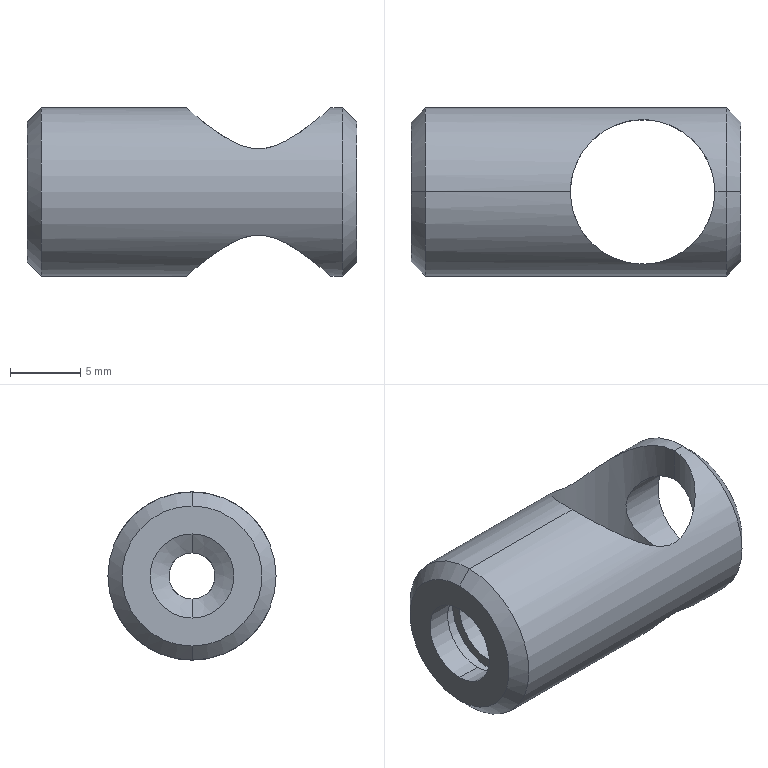Part | SolidWorks | features BaseBody 1 | 1 solid | 24 faces | box 23.5 x 12 x 12 mm | volume 1412 mm3 | cylinder 14 | cone 6 | plane 4 | commonest cylinder face diameters 6 x4 3.3 x2 7 x2 7.4 x2 10.3 x2 12 x2
STEP:
#1=CARTESIAN_POINT('',(486.537,37.715,59.366));
#2=VERTEX_POINT('',#1);
#3=CARTESIAN_POINT('',(486.537,37.715,71.366));
#4=VERTEX_POINT('',#3);
#5=CARTESIAN_POINT('',(486.537,37.715,65.366));
#6=DIRECTION('',(1.,0.,0.000000013));
#7=DIRECTION('',(0.,1.,0.));
#8=AXIS2_PLACEMENT_3D('',#5,#6,#7);
#9=CIRCLE('',#8,6.);
#10=EDGE_CURVE('',#2,#4,#9,.T.);
#11=ORIENTED_EDGE('',*,*,#10,.F.);
#12=CARTESIAN_POINT('',(485.687,37.715,59.366));
#13=VERTEX_POINT('',#12);
#14=CARTESIAN_POINT('',(486.537,37.715,59.366));
#15=DIRECTION('',(-1.,0.,-0.000000013));
#16=VECTOR('',#15,1000.);
#17=LINE('',#14,#16);
#18=EDGE_CURVE('',#2,#13,#17,.T.);
#19=ORIENTED_EDGE('',*,*,#18,.T.);
#20=CARTESIAN_POINT('',(475.387,37.715,59.366));
#21=VERTEX_POINT('',#20);
#22=CARTESIAN_POINT('',(475.387,37.715,59.366));
#23=CARTESIAN_POINT('',(475.387,37.895,59.366));
#24=CARTESIAN_POINT('',(475.396,38.075,59.374));
#25=CARTESIAN_POINT('',(475.434,38.436,59.407));
#26=CARTESIAN_POINT('',(475.463,38.616,59.431));
#27=CARTESIAN_POINT('',(475.538,38.965,59.495));
#28=CARTESIAN_POINT('',(475.584,39.136,59.534));
#29=CARTESIAN_POINT('',(475.692,39.47,59.626));
#30=CARTESIAN_POINT('',(475.755,39.634,59.679));
#31=CARTESIAN_POINT('',(475.964,40.108,59.854));
#32=CARTESIAN_POINT('',(476.129,40.399,59.991));
#33=CARTESIAN_POINT('',(476.509,40.941,60.297));
#34=CARTESIAN_POINT('',(476.72,41.187,60.465));
#35=CARTESIAN_POINT('',(477.174,41.628,60.809));
#36=CARTESIAN_POINT('',(477.418,41.825,60.988));
#37=CARTESIAN_POINT('',(477.945,42.176,61.346));
#38=CARTESIAN_POINT('',(478.225,42.328,61.524));
#39=CARTESIAN_POINT('',(478.67,42.517,61.768));
#40=CARTESIAN_POINT('',(478.824,42.574,61.846));
#41=CARTESIAN_POINT('',(479.142,42.675,61.989));
#42=CARTESIAN_POINT('',(479.309,42.719,62.055));
#43=CARTESIAN_POINT('',(479.647,42.79,62.165));
#44=CARTESIAN_POINT('',(479.821,42.818,62.21));
#45=CARTESIAN_POINT('',(480.178,42.855,62.272));
#46=CARTESIAN_POINT('',(480.362,42.865,62.288));
#47=CARTESIAN_POINT('',(480.913,42.864,62.286));
#48=CARTESIAN_POINT('',(481.268,42.824,62.218));
#49=CARTESIAN_POINT('',(481.949,42.679,61.994));
#50=CARTESIAN_POINT('',(482.263,42.578,61.845));
#51=CARTESIAN_POINT('',(482.858,42.323,61.518));
#52=CARTESIAN_POINT('',(483.139,42.17,61.34));
#53=CARTESIAN_POINT('',(483.66,41.822,60.985));
#54=CARTESIAN_POINT('',(483.903,41.625,60.807));
#55=CARTESIAN_POINT('',(484.358,41.182,60.461));
#56=CARTESIAN_POINT('',(484.57,40.933,60.293));
#57=CARTESIAN_POINT('',(484.946,40.396,59.99));
#58=CARTESIAN_POINT('',(485.111,40.106,59.853));
#59=CARTESIAN_POINT('',(485.39,39.471,59.619));
#60=CARTESIAN_POINT('',(485.499,39.139,59.527));
#61=CARTESIAN_POINT('',(485.611,38.615,59.431));
#62=CARTESIAN_POINT('',(485.639,38.435,59.407));
#63=CARTESIAN_POINT('',(485.677,38.075,59.374));
#64=CARTESIAN_POINT('',(485.687,37.895,59.366));
#65=CARTESIAN_POINT('',(485.687,37.715,59.366));
#66=B_SPLINE_CURVE_WITH_KNOTS('',3,(#22,#23,#24,#25,#26,#27,#28,#29,#30,#31,#32,#33,#34,#35,#36,#37,#38,#39,#40,#41,#42,#43,#44,#45,#46,#47,#48,#49,#50,#51,#52,#53,#54,#55,#56,#57,#58,#59,#60,#61,#62,#63,#64,#65),.UNSPECIFIED.,.F.,.F.,(4,2,2,2,2,2,2,2,2,2,2,2,2,2,2,2,2,2,2,2,2,4),(0.008683,0.009225,0.009768,0.01031,0.01085,0.01194,0.01302,0.01411,0.01519,0.01573,0.01627,0.01682,0.01736,0.01844,0.01953,0.02061,0.0217,0.02278,0.02387,0.02495,0.02549,0.02604),.UNSPECIFIED.);
#67=EDGE_CURVE('',#21,#13,#66,.T.);
#68=ORIENTED_EDGE('',*,*,#67,.F.);
#69=CARTESIAN_POINT('',(465.037,37.715,59.366));
#70=VERTEX_POINT('',#69);
#71=CARTESIAN_POINT('',(486.537,37.715,59.366));
#72=DIRECTION('',(-1.,0.,-0.000000013));
#73=VECTOR('',#72,1000.);
#74=LINE('',#71,#73);
#75=EDGE_CURVE('',#21,#70,#74,.T.);
#76=ORIENTED_EDGE('',*,*,#75,.T.);
#77=CARTESIAN_POINT('',(465.037,37.715,71.366));
#78=VERTEX_POINT('',#77);
#79=CARTESIAN_POINT('',(465.037,37.715,65.366));
#80=DIRECTION('',(-1.,0.,-0.000000013));
#81=DIRECTION('',(0.,1.,0.));
#82=AXIS2_PLACEMENT_3D('',#79,#80,#81);
#83=CIRCLE('',#82,6.);
#84=EDGE_CURVE('',#78,#70,#83,.T.);
#85=ORIENTED_EDGE('',*,*,#84,.F.);
#86=CARTESIAN_POINT('',(475.387,37.715,71.366));
#87=VERTEX_POINT('',#86);
#88=CARTESIAN_POINT('',(486.537,37.715,71.366));
#89=DIRECTION('',(-1.,0.,-0.000000013));
#90=VECTOR('',#89,1000.);
#91=LINE('',#88,#90);
#92=EDGE_CURVE('',#87,#78,#91,.T.);
#93=ORIENTED_EDGE('',*,*,#92,.F.);
#94=CARTESIAN_POINT('',(485.687,37.715,71.366));
#95=VERTEX_POINT('',#94);
#96=CARTESIAN_POINT('',(485.687,37.715,71.366));
#97=CARTESIAN_POINT('',(485.687,37.895,71.366));
#98=CARTESIAN_POINT('',(485.677,38.075,71.358));
#99=CARTESIAN_POINT('',(485.639,38.436,71.325));
#100=CARTESIAN_POINT('',(485.611,38.616,71.301));
#101=CARTESIAN_POINT('',(485.536,38.965,71.237));
#102=CARTESIAN_POINT('',(485.49,39.136,71.198));
#103=CARTESIAN_POINT('',(485.382,39.47,71.106));
#104=CARTESIAN_POINT('',(485.319,39.634,71.053));
#105=CARTESIAN_POINT('',(485.11,40.108,70.878));
#106=CARTESIAN_POINT('',(484.944,40.399,70.741));
#107=CARTESIAN_POINT('',(484.565,40.941,70.435));
#108=CARTESIAN_POINT('',(484.354,41.187,70.267));
#109=CARTESIAN_POINT('',(483.9,41.628,69.923));
#110=CARTESIAN_POINT('',(483.656,41.825,69.744));
#111=CARTESIAN_POINT('',(483.129,42.176,69.386));
#112=CARTESIAN_POINT('',(482.849,42.328,69.208));
#113=CARTESIAN_POINT('',(482.403,42.517,68.964));
#114=CARTESIAN_POINT('',(482.25,42.574,68.886));
#115=CARTESIAN_POINT('',(481.931,42.675,68.743));
#116=CARTESIAN_POINT('',(481.765,42.719,68.677));
#117=CARTESIAN_POINT('',(481.426,42.79,68.566));
#118=CARTESIAN_POINT('',(481.253,42.818,68.522));
#119=CARTESIAN_POINT('',(480.896,42.855,68.46));
#120=CARTESIAN_POINT('',(480.712,42.865,68.444));
#121=CARTESIAN_POINT('',(480.16,42.864,68.446));
#122=CARTESIAN_POINT('',(479.805,42.824,68.514));
#123=CARTESIAN_POINT('',(479.124,42.679,68.738));
#124=CARTESIAN_POINT('',(478.811,42.578,68.886));
#125=CARTESIAN_POINT('',(478.216,42.323,69.213));
#126=CARTESIAN_POINT('',(477.935,42.17,69.392));
#127=CARTESIAN_POINT('',(477.414,41.822,69.747));
#128=CARTESIAN_POINT('',(477.171,41.625,69.925));
#129=CARTESIAN_POINT('',(476.715,41.182,70.271));
#130=CARTESIAN_POINT('',(476.503,40.933,70.439));
#131=CARTESIAN_POINT('',(476.128,40.396,70.742));
#132=CARTESIAN_POINT('',(475.962,40.106,70.879));
#133=CARTESIAN_POINT('',(475.683,39.471,71.113));
#134=CARTESIAN_POINT('',(475.575,39.139,71.205));
#135=CARTESIAN_POINT('',(475.463,38.615,71.301));
#136=CARTESIAN_POINT('',(475.434,38.435,71.325));
#137=CARTESIAN_POINT('',(475.396,38.075,71.358));
#138=CARTESIAN_POINT('',(475.387,37.895,71.366));
#139=CARTESIAN_POINT('',(475.387,37.715,71.366));
#140=B_SPLINE_CURVE_WITH_KNOTS('',3,(#96,#97,#98,#99,#100,#101,#102,#103,#104,#105,#106,#107,#108,#109,#110,#111,#112,#113,#114,#115,#116,#117,#118,#119,#120,#121,#122,#123,#124,#125,#126,#127,#128,#129,#130,#131,#132,#133,#134,#135,#136,#137,#138,#139),.UNSPECIFIED.,.F.,.F.,(4,2,2,2,2,2,2,2,2,2,2,2,2,2,2,2,2,2,2,2,2,4),(0.008683,0.009225,0.009768,0.01031,0.01085,0.01194,0.01302,0.01411,0.01519,0.01573,0.01627,0.01682,0.01736,0.01844,0.01953,0.02061,0.0217,0.02278,0.02387,0.02495,0.02549,0.02604),.UNSPECIFIED.);
#141=EDGE_CURVE('',#95,#87,#140,.T.);
#142=ORIENTED_EDGE('',*,*,#141,.F.);
#143=CARTESIAN_POINT('',(486.537,37.715,71.366));
#144=DIRECTION('',(-1.,0.,-0.000000013));
#145=VECTOR('',#144,1000.);
#146=LINE('',#143,#145);
#147=EDGE_CURVE('',#4,#95,#146,.T.);
#148=ORIENTED_EDGE('',*,*,#147,.F.);
#149=EDGE_LOOP('',(#11,#19,#68,#76,#85,#93,#142,#148));
#150=FACE_OUTER_BOUND('',#149,.T.);
#151=CARTESIAN_POINT('',(486.537,37.715,65.366));
#152=DIRECTION('',(-1.,0.,-0.000000013));
#153=DIRECTION('',(-0.000000013,0.,1.));
#154=AXIS2_PLACEMENT_3D('',#151,#152,#153);
#155=CYLINDRICAL_SURFACE('',#154,6.);
#156=ADVANCED_FACE('',(#150),#155,.T.);
#157=CARTESIAN_POINT('',(487.537,37.715,60.366));
#158=VERTEX_POINT('',#157);
#159=CARTESIAN_POINT('',(487.537,37.715,70.366));
#160=VERTEX_POINT('',#159);
#161=CARTESIAN_POINT('',(487.537,37.715,65.366));
#162=DIRECTION('',(1.,0.,0.000000013));
#163=DIRECTION('',(-0.000000013,0.,1.));
#164=AXIS2_PLACEMENT_3D('',#161,#162,#163);
#165=CIRCLE('',#164,5.);
#166=EDGE_CURVE('',#158,#160,#165,.T.);
#167=ORIENTED_EDGE('',*,*,#166,.F.);
#168=CARTESIAN_POINT('',(487.537,37.715,60.366));
#169=DIRECTION('',(-0.7071,0.,-0.7071));
#170=VECTOR('',#169,1000.);
#171=LINE('',#168,#170);
#172=EDGE_CURVE('',#158,#2,#171,.T.);
#173=ORIENTED_EDGE('',*,*,#172,.T.);
#174=ORIENTED_EDGE('',*,*,#10,.T.);
#175=CARTESIAN_POINT('',(487.537,37.715,70.366));
#176=DIRECTION('',(-0.7071,0.,0.7071));
#177=VECTOR('',#176,1000.);
#178=LINE('',#175,#177);
#179=EDGE_CURVE('',#160,#4,#178,.T.);
#180=ORIENTED_EDGE('',*,*,#179,.F.);
#181=EDGE_LOOP('',(#167,#173,#174,#180));
#182=FACE_OUTER_BOUND('',#181,.T.);
#183=CARTESIAN_POINT('',(487.537,37.715,65.366));
#184=DIRECTION('',(-1.,0.,-0.000000013));
#185=DIRECTION('',(-0.000000013,0.,1.));
#186=AXIS2_PLACEMENT_3D('',#183,#184,#185);
#187=CONICAL_SURFACE('',#186,5.,0.7854);
#188=ADVANCED_FACE('',(#182),#187,.T.);
#189=CARTESIAN_POINT('',(464.037,37.715,70.366));
#190=VERTEX_POINT('',#189);
#191=CARTESIAN_POINT('',(464.037,37.715,60.366));
#192=VERTEX_POINT('',#191);
#193=CARTESIAN_POINT('',(464.037,37.715,65.366));
#194=DIRECTION('',(-1.,0.,-0.000000013));
#195=DIRECTION('',(0.000000013,0.,-1.));
#196=AXIS2_PLACEMENT_3D('',#193,#194,#195);
#197=CIRCLE('',#196,5.);
#198=EDGE_CURVE('',#190,#192,#197,.T.);
#199=ORIENTED_EDGE('',*,*,#198,.F.);
#200=CARTESIAN_POINT('',(465.037,37.715,71.366));
#201=DIRECTION('',(0.7071,0.,0.7071));
#202=VECTOR('',#201,1000.);
#203=LINE('',#200,#202);
#204=EDGE_CURVE('',#190,#78,#203,.T.);
#205=ORIENTED_EDGE('',*,*,#204,.T.);
#206=ORIENTED_EDGE('',*,*,#84,.T.);
#207=CARTESIAN_POINT('',(465.037,37.715,59.366));
#208=DIRECTION('',(0.7071,0.,-0.7071));
#209=VECTOR('',#208,1000.);
#210=LINE('',#207,#209);
#211=EDGE_CURVE('',#192,#70,#210,.T.);
#212=ORIENTED_EDGE('',*,*,#211,.F.);
#213=EDGE_LOOP('',(#199,#205,#206,#212));
#214=FACE_OUTER_BOUND('',#213,.T.);
#215=CARTESIAN_POINT('',(465.037,37.715,65.366));
#216=DIRECTION('',(1.,0.,0.000000013));
#217=DIRECTION('',(0.000000013,0.,-1.));
#218=AXIS2_PLACEMENT_3D('',#215,#216,#217);
#219=CONICAL_SURFACE('',#218,6.,0.7854);
#220=ADVANCED_FACE('',(#214),#219,.T.);
#221=CARTESIAN_POINT('',(485.687,37.715,59.366));
#222=CARTESIAN_POINT('',(485.687,37.535,59.366));
#223=CARTESIAN_POINT('',(485.677,37.354,59.374));
#224=CARTESIAN_POINT('',(485.639,36.993,59.407));
#225=CARTESIAN_POINT('',(485.611,36.814,59.431));
#226=CARTESIAN_POINT('',(485.536,36.465,59.495));
#227=CARTESIAN_POINT('',(485.49,36.294,59.534));
#228=CARTESIAN_POINT('',(485.382,35.96,59.626));
#229=CARTESIAN_POINT('',(485.319,35.796,59.679));
#230=CARTESIAN_POINT('',(485.11,35.322,59.853));
#231=CARTESIAN_POINT('',(484.945,35.031,59.991));
#232=CARTESIAN_POINT('',(484.565,34.489,60.297));
#233=CARTESIAN_POINT('',(484.354,34.243,60.464));
#234=CARTESIAN_POINT('',(483.901,33.802,60.809));
#235=CARTESIAN_POINT('',(483.657,33.605,60.987));
#236=CARTESIAN_POINT('',(483.13,33.254,61.345));
#237=CARTESIAN_POINT('',(482.85,33.102,61.523));
#238=CARTESIAN_POINT('',(482.405,32.913,61.767));
#239=CARTESIAN_POINT('',(482.251,32.856,61.845));
#240=CARTESIAN_POINT('',(481.933,32.755,61.989));
#241=CARTESIAN_POINT('',(481.767,32.711,62.055));
#242=CARTESIAN_POINT('',(481.428,32.639,62.165));
#243=CARTESIAN_POINT('',(481.255,32.612,62.21));
#244=CARTESIAN_POINT('',(480.898,32.574,62.271));
#245=CARTESIAN_POINT('',(480.714,32.564,62.288));
#246=CARTESIAN_POINT('',(480.162,32.565,62.287));
#247=CARTESIAN_POINT('',(479.807,32.605,62.219));
#248=CARTESIAN_POINT('',(479.126,32.75,61.995));
#249=CARTESIAN_POINT('',(478.813,32.851,61.846));
#250=CARTESIAN_POINT('',(478.217,33.105,61.519));
#251=CARTESIAN_POINT('',(477.936,33.259,61.34));
#252=CARTESIAN_POINT('',(477.415,33.607,60.985));
#253=CARTESIAN_POINT('',(477.171,33.804,60.807));
#254=CARTESIAN_POINT('',(476.716,34.247,60.461));
#255=CARTESIAN_POINT('',(476.504,34.495,60.293));
#256=CARTESIAN_POINT('',(476.128,35.033,59.99));
#257=CARTESIAN_POINT('',(475.963,35.323,59.853));
#258=CARTESIAN_POINT('',(475.683,35.958,59.619));
#259=CARTESIAN_POINT('',(475.575,36.29,59.527));
#260=CARTESIAN_POINT('',(475.463,36.814,59.431));
#261=CARTESIAN_POINT('',(475.434,36.994,59.407));
#262=CARTESIAN_POINT('',(475.396,37.354,59.374));
#263=CARTESIAN_POINT('',(475.387,37.534,59.366));
#264=CARTESIAN_POINT('',(475.387,37.715,59.366));
#265=B_SPLINE_CURVE_WITH_KNOTS('',3,(#221,#222,#223,#224,#225,#226,#227,#228,#229,#230,#231,#232,#233,#234,#235,#236,#237,#238,#239,#240,#241,#242,#243,#244,#245,#246,#247,#248,#249,#250,#251,#252,#253,#254,#255,#256,#257,#258,#259,#260,#261,#262,#263,#264),.UNSPECIFIED.,.F.,.F.,(4,2,2,2,2,2,2,2,2,2,2,2,2,2,2,2,2,2,2,2,2,4),(0.02604,0.02658,0.02712,0.02766,0.0282,0.02929,0.03037,0.03146,0.03254,0.03309,0.03363,0.03417,0.03471,0.0358,0.03688,0.03797,0.03905,0.04013,0.04122,0.0423,0.04285,0.04339),.UNSPECIFIED.);
#266=EDGE_CURVE('',#13,#21,#265,.T.);
#267=ORIENTED_EDGE('',*,*,#266,.T.);
#268=CARTESIAN_POINT('',(475.387,37.715,63.716));
#269=VERTEX_POINT('',#268);
#270=CARTESIAN_POINT('',(475.387,37.715,59.293));
#271=DIRECTION('',(-0.000000013,0.,1.));
#272=VECTOR('',#271,1000.);
#273=LINE('',#270,#272);
#274=EDGE_CURVE('',#21,#269,#273,.T.);
#275=ORIENTED_EDGE('',*,*,#274,.T.);
#276=CARTESIAN_POINT('',(475.387,37.715,67.016));
#277=VERTEX_POINT('',#276);
#278=CARTESIAN_POINT('',(475.387,37.715,63.716));
#279=CARTESIAN_POINT('',(475.387,37.606,63.716));
#280=CARTESIAN_POINT('',(475.39,37.496,63.727));
#281=CARTESIAN_POINT('',(475.404,37.284,63.769));
#282=CARTESIAN_POINT('',(475.414,37.181,63.801));
#283=CARTESIAN_POINT('',(475.451,36.88,63.926));
#284=CARTESIAN_POINT('',(475.486,36.699,64.048));
#285=CARTESIAN_POINT('',(475.539,36.471,64.276));
#286=CARTESIAN_POINT('',(475.556,36.403,64.359));
#287=CARTESIAN_POINT('',(475.589,36.284,64.537));
#288=CARTESIAN_POINT('',(475.605,36.232,64.633));
#289=CARTESIAN_POINT('',(475.643,36.109,64.931));
#290=CARTESIAN_POINT('',(475.658,36.064,65.148));
#291=CARTESIAN_POINT('',(475.658,36.065,65.477));
#292=CARTESIAN_POINT('',(475.655,36.076,65.585));
#293=CARTESIAN_POINT('',(475.64,36.118,65.797));
#294=CARTESIAN_POINT('',(475.63,36.15,65.902));
#295=CARTESIAN_POINT('',(475.604,36.234,66.101));
#296=CARTESIAN_POINT('',(475.589,36.284,66.196));
#297=CARTESIAN_POINT('',(475.556,36.404,66.374));
#298=CARTESIAN_POINT('',(475.538,36.473,66.458));
#299=CARTESIAN_POINT('',(475.485,36.7,66.685));
#300=CARTESIAN_POINT('',(475.451,36.883,66.807));
#301=CARTESIAN_POINT('',(475.414,37.181,66.931));
#302=CARTESIAN_POINT('',(475.404,37.285,66.963));
#303=CARTESIAN_POINT('',(475.39,37.499,67.005));
#304=CARTESIAN_POINT('',(475.387,37.606,67.016));
#305=CARTESIAN_POINT('',(475.387,37.715,67.016));
#306=B_SPLINE_CURVE_WITH_KNOTS('',3,(#278,#279,#280,#281,#282,#283,#284,#285,#286,#287,#288,#289,#290,#291,#292,#293,#294,#295,#296,#297,#298,#299,#300,#301,#302,#303,#304,#305),.UNSPECIFIED.,.F.,.F.,(4,2,2,2,2,2,2,2,2,2,2,2,2,4),(0.002597,0.002922,0.003246,0.003895,0.004219,0.004544,0.005193,0.005517,0.005842,0.006166,0.00649,0.007139,0.007464,0.007788),.UNSPECIFIED.);
#307=EDGE_CURVE('',#269,#277,#306,.T.);
#308=ORIENTED_EDGE('',*,*,#307,.T.);
#309=CARTESIAN_POINT('',(475.387,37.715,59.293));
#310=DIRECTION('',(-0.000000013,0.,1.));
#311=VECTOR('',#310,1000.);
#312=LINE('',#309,#311);
#313=EDGE_CURVE('',#277,#87,#312,.T.);
#314=ORIENTED_EDGE('',*,*,#313,.T.);
#315=CARTESIAN_POINT('',(475.387,37.715,71.366));
#316=CARTESIAN_POINT('',(475.387,37.535,71.366));
#317=CARTESIAN_POINT('',(475.396,37.354,71.358));
#318=CARTESIAN_POINT('',(475.434,36.993,71.325));
#319=CARTESIAN_POINT('',(475.463,36.814,71.301));
#320=CARTESIAN_POINT('',(475.538,36.465,71.237));
#321=CARTESIAN_POINT('',(475.584,36.294,71.198));
#322=CARTESIAN_POINT('',(475.692,35.96,71.106));
#323=CARTESIAN_POINT('',(475.754,35.796,71.053));
#324=CARTESIAN_POINT('',(475.963,35.322,70.879));
#325=CARTESIAN_POINT('',(476.129,35.031,70.741));
#326=CARTESIAN_POINT('',(476.508,34.489,70.435));
#327=CARTESIAN_POINT('',(476.719,34.243,70.268));
#328=CARTESIAN_POINT('',(477.173,33.802,69.923));
#329=CARTESIAN_POINT('',(477.417,33.605,69.745));
#330=CARTESIAN_POINT('',(477.944,33.254,69.386));
#331=CARTESIAN_POINT('',(478.224,33.102,69.209));
#332=CARTESIAN_POINT('',(478.669,32.913,68.965));
#333=CARTESIAN_POINT('',(478.822,32.856,68.887));
#334=CARTESIAN_POINT('',(479.141,32.755,68.743));
#335=CARTESIAN_POINT('',(479.307,32.711,68.677));
#336=CARTESIAN_POINT('',(479.645,32.639,68.567));
#337=CARTESIAN_POINT('',(479.819,32.612,68.522));
#338=CARTESIAN_POINT('',(480.176,32.574,68.461));
#339=CARTESIAN_POINT('',(480.36,32.564,68.444));
#340=CARTESIAN_POINT('',(480.911,32.565,68.445));
#341=CARTESIAN_POINT('',(481.266,32.605,68.513));
#342=CARTESIAN_POINT('',(481.948,32.75,68.737));
#343=CARTESIAN_POINT('',(482.261,32.851,68.886));
#344=CARTESIAN_POINT('',(482.857,33.105,69.213));
#345=CARTESIAN_POINT('',(483.138,33.259,69.391));
#346=CARTESIAN_POINT('',(483.659,33.607,69.746));
#347=CARTESIAN_POINT('',(483.902,33.804,69.925));
#348=CARTESIAN_POINT('',(484.358,34.247,70.27));
#349=CARTESIAN_POINT('',(484.57,34.495,70.439));
#350=CARTESIAN_POINT('',(484.945,35.033,70.742));
#351=CARTESIAN_POINT('',(485.111,35.323,70.879));
#352=CARTESIAN_POINT('',(485.39,35.958,71.113));
#353=CARTESIAN_POINT('',(485.499,36.29,71.205));
#354=CARTESIAN_POINT('',(485.611,36.814,71.301));
#355=CARTESIAN_POINT('',(485.639,36.994,71.325));
#356=CARTESIAN_POINT('',(485.677,37.354,71.358));
#357=CARTESIAN_POINT('',(485.687,37.534,71.366));
#358=CARTESIAN_POINT('',(485.687,37.715,71.366));
#359=B_SPLINE_CURVE_WITH_KNOTS('',3,(#315,#316,#317,#318,#319,#320,#321,#322,#323,#324,#325,#326,#327,#328,#329,#330,#331,#332,#333,#334,#335,#336,#337,#338,#339,#340,#341,#342,#343,#344,#345,#346,#347,#348,#349,#350,#351,#352,#353,#354,#355,#356,#357,#358),.UNSPECIFIED.,.F.,.F.,(4,2,2,2,2,2,2,2,2,2,2,2,2,2,2,2,2,2,2,2,2,4),(0.02604,0.02658,0.02712,0.02766,0.0282,0.02929,0.03037,0.03146,0.03254,0.03309,0.03363,0.03417,0.03471,0.0358,0.03688,0.03797,0.03905,0.04013,0.04122,0.0423,0.04285,0.04339),.UNSPECIFIED.);
#360=EDGE_CURVE('',#87,#95,#359,.T.);
#361=ORIENTED_EDGE('',*,*,#360,.T.);
#362=CARTESIAN_POINT('',(485.687,37.715,68.866));
#363=VERTEX_POINT('',#362);
#364=CARTESIAN_POINT('',(485.687,37.715,59.293));
#365=DIRECTION('',(-0.000000013,0.,1.));
#366=VECTOR('',#365,1000.);
#367=LINE('',#364,#366);
#368=EDGE_CURVE('',#363,#95,#367,.T.);
#369=ORIENTED_EDGE('',*,*,#368,.F.);
#370=CARTESIAN_POINT('',(485.687,37.715,61.866));
#371=VERTEX_POINT('',#370);
#372=CARTESIAN_POINT('',(485.687,37.715,68.866));
#373=CARTESIAN_POINT('',(485.687,37.476,68.866));
#374=CARTESIAN_POINT('',(485.67,37.242,68.842));
#375=CARTESIAN_POINT('',(485.607,36.78,68.747));
#376=CARTESIAN_POINT('',(485.559,36.555,68.676));
#377=CARTESIAN_POINT('',(485.442,36.132,68.496));
#378=CARTESIAN_POINT('',(485.372,35.93,68.385));
#379=CARTESIAN_POINT('',(485.218,35.558,68.132));
#380=CARTESIAN_POINT('',(485.135,35.388,67.99));
#381=CARTESIAN_POINT('',(484.962,35.074,67.674));
#382=CARTESIAN_POINT('',(484.874,34.934,67.502));
#383=CARTESIAN_POINT('',(484.706,34.687,67.136));
#384=CARTESIAN_POINT('',(484.625,34.58,66.94));
#385=CARTESIAN_POINT('',(484.482,34.402,66.519));
#386=CARTESIAN_POINT('',(484.422,34.334,66.3));
#387=CARTESIAN_POINT('',(484.338,34.239,65.842));
#388=CARTESIAN_POINT('',(484.314,34.214,65.602));
#389=CARTESIAN_POINT('',(484.315,34.215,65.122));
#390=CARTESIAN_POINT('',(484.338,34.24,64.888));
#391=CARTESIAN_POINT('',(484.422,34.334,64.432));
#392=CARTESIAN_POINT('',(484.483,34.404,64.208));
#393=CARTESIAN_POINT('',(484.625,34.581,63.792));
#394=CARTESIAN_POINT('',(484.706,34.688,63.594));
#395=CARTESIAN_POINT('',(484.876,34.937,63.225));
#396=CARTESIAN_POINT('',(484.964,35.077,63.055));
#397=CARTESIAN_POINT('',(485.135,35.389,62.741));
#398=CARTESIAN_POINT('',(485.22,35.563,62.597));
#399=CARTESIAN_POINT('',(485.373,35.932,62.345));
#400=CARTESIAN_POINT('',(485.442,36.129,62.237));
#401=CARTESIAN_POINT('',(485.559,36.551,62.057));
#402=CARTESIAN_POINT('',(485.606,36.778,61.986));
#403=CARTESIAN_POINT('',(485.67,37.238,61.891));
#404=CARTESIAN_POINT('',(485.687,37.476,61.866));
#405=CARTESIAN_POINT('',(485.687,37.715,61.866));
#406=B_SPLINE_CURVE_WITH_KNOTS('',3,(#372,#373,#374,#375,#376,#377,#378,#379,#380,#381,#382,#383,#384,#385,#386,#387,#388,#389,#390,#391,#392,#393,#394,#395,#396,#397,#398,#399,#400,#401,#402,#403,#404,#405),.UNSPECIFIED.,.F.,.F.,(4,2,2,2,2,2,2,2,2,2,2,2,2,2,2,2,4),(0.005665,0.006372,0.007079,0.007786,0.008493,0.0092,0.009907,0.01061,0.01132,0.01203,0.01273,0.01344,0.01415,0.01486,0.01556,0.01627,0.01698),.UNSPECIFIED.);
#407=EDGE_CURVE('',#363,#371,#406,.T.);
#408=ORIENTED_EDGE('',*,*,#407,.T.);
#409=CARTESIAN_POINT('',(485.687,37.715,59.293));
#410=DIRECTION('',(-0.000000013,0.,1.));
#411=VECTOR('',#410,1000.);
#412=LINE('',#409,#411);
#413=EDGE_CURVE('',#13,#371,#412,.T.);
#414=ORIENTED_EDGE('',*,*,#413,.F.);
#415=EDGE_LOOP('',(#267,#275,#308,#314,#361,#369,#408,#414));
#416=FACE_OUTER_BOUND('',#415,.T.);
#417=CARTESIAN_POINT('',(480.537,37.715,59.293));
#418=DIRECTION('',(-0.000000013,0.,1.));
#419=DIRECTION('',(1.,0.,0.000000013));
#420=AXIS2_PLACEMENT_3D('',#417,#418,#419);
#421=CYLINDRICAL_SURFACE('',#420,5.15);
#422=ADVANCED_FACE('',(#416),#421,.F.);
#423=CARTESIAN_POINT('',(470.316,37.715,63.716));
#424=VERTEX_POINT('',#423);
#425=CARTESIAN_POINT('',(470.316,37.715,67.016));
#426=VERTEX_POINT('',#425);
#427=CARTESIAN_POINT('',(470.316,37.715,65.366));
#428=DIRECTION('',(-1.,0.,-0.000000013));
#429=DIRECTION('',(0.,1.,0.));
#430=AXIS2_PLACEMENT_3D('',#427,#428,#429);
#431=CIRCLE('',#430,1.65);
#432=EDGE_CURVE('',#424,#426,#431,.T.);
#433=ORIENTED_EDGE('',*,*,#432,.T.);
#434=CARTESIAN_POINT('',(470.316,37.715,67.016));
#435=DIRECTION('',(1.,0.,0.000000013));
#436=VECTOR('',#435,1000.);
#437=LINE('',#434,#436);
#438=EDGE_CURVE('',#426,#277,#437,.T.);
#439=ORIENTED_EDGE('',*,*,#438,.T.);
#440=ORIENTED_EDGE('',*,*,#307,.F.);
#441=CARTESIAN_POINT('',(470.316,37.715,63.716));
#442=DIRECTION('',(1.,0.,0.000000013));
#443=VECTOR('',#442,1000.);
#444=LINE('',#441,#443);
#445=EDGE_CURVE('',#424,#269,#444,.T.);
#446=ORIENTED_EDGE('',*,*,#445,.F.);
#447=EDGE_LOOP('',(#433,#439,#440,#446));
#448=FACE_OUTER_BOUND('',#447,.T.);
#449=CARTESIAN_POINT('',(470.316,37.715,65.366));
#450=DIRECTION('',(1.,0.,0.000000013));
#451=DIRECTION('',(0.000000013,0.,-1.));
#452=AXIS2_PLACEMENT_3D('',#449,#450,#451);
#453=CYLINDRICAL_SURFACE('',#452,1.65);
#454=ADVANCED_FACE('',(#448),#453,.F.);
#455=ORIENTED_EDGE('',*,*,#407,.F.);
#456=CARTESIAN_POINT('',(487.537,37.715,68.866));
#457=VERTEX_POINT('',#456);
#458=CARTESIAN_POINT('',(484.295,37.715,68.866));
#459=DIRECTION('',(1.,0.,0.000000013));
#460=VECTOR('',#459,1000.);
#461=LINE('',#458,#460);
#462=EDGE_CURVE('',#363,#457,#461,.T.);
#463=ORIENTED_EDGE('',*,*,#462,.T.);
#464=CARTESIAN_POINT('',(487.537,37.715,61.866));
#465=VERTEX_POINT('',#464);
#466=CARTESIAN_POINT('',(487.537,37.715,65.366));
#467=DIRECTION('',(1.,0.,0.000000013));
#468=DIRECTION('',(0.000000013,0.,-1.));
#469=AXIS2_PLACEMENT_3D('',#466,#467,#468);
#470=CIRCLE('',#469,3.5);
#471=EDGE_CURVE('',#457,#465,#470,.T.);
#472=ORIENTED_EDGE('',*,*,#471,.T.);
#473=CARTESIAN_POINT('',(484.295,37.715,61.866));
#474=DIRECTION('',(1.,0.,0.000000013));
#475=VECTOR('',#474,1000.);
#476=LINE('',#473,#475);
#477=EDGE_CURVE('',#371,#465,#476,.T.);
#478=ORIENTED_EDGE('',*,*,#477,.F.);
#479=EDGE_LOOP('',(#455,#463,#472,#478));
#480=FACE_OUTER_BOUND('',#479,.T.);
#481=CARTESIAN_POINT('',(484.295,37.715,65.366));
#482=DIRECTION('',(1.,0.,0.000000013));
#483=DIRECTION('',(0.000000013,0.,-1.));
#484=AXIS2_PLACEMENT_3D('',#481,#482,#483);
#485=CYLINDRICAL_SURFACE('',#484,3.5);
#486=ADVANCED_FACE('',(#480),#485,.F.);
#487=CARTESIAN_POINT('',(465.837,37.715,68.366));
#488=VERTEX_POINT('',#487);
#489=CARTESIAN_POINT('',(465.837,37.715,62.366));
#490=VERTEX_POINT('',#489);
#491=CARTESIAN_POINT('',(465.837,37.715,65.366));
#492=DIRECTION('',(1.,0.,0.000000013));
#493=DIRECTION('',(-0.000000013,0.,1.));
#494=AXIS2_PLACEMENT_3D('',#491,#492,#493);
#495=CIRCLE('',#494,3.);
#496=EDGE_CURVE('',#488,#490,#495,.T.);
#497=ORIENTED_EDGE('',*,*,#496,.T.);
#498=CARTESIAN_POINT('',(464.037,37.715,62.366));
#499=VERTEX_POINT('',#498);
#500=CARTESIAN_POINT('',(465.837,37.715,62.366));
#501=DIRECTION('',(-1.,0.,-0.000000013));
#502=VECTOR('',#501,1000.);
#503=LINE('',#500,#502);
#504=EDGE_CURVE('',#490,#499,#503,.T.);
#505=ORIENTED_EDGE('',*,*,#504,.T.);
#506=CARTESIAN_POINT('',(464.037,37.715,68.366));
#507=VERTEX_POINT('',#506);
#508=CARTESIAN_POINT('',(464.037,37.715,65.366));
#509=DIRECTION('',(1.,0.,0.000000013));
#510=DIRECTION('',(-0.000000013,0.,1.));
#511=AXIS2_PLACEMENT_3D('',#508,#509,#510);
#512=CIRCLE('',#511,3.);
#513=EDGE_CURVE('',#507,#499,#512,.T.);
#514=ORIENTED_EDGE('',*,*,#513,.F.);
#515=CARTESIAN_POINT('',(465.837,37.715,68.366));
#516=DIRECTION('',(-1.,0.,-0.000000013));
#517=VECTOR('',#516,1000.);
#518=LINE('',#515,#517);
#519=EDGE_CURVE('',#488,#507,#518,.T.);
#520=ORIENTED_EDGE('',*,*,#519,.F.);
#521=EDGE_LOOP('',(#497,#505,#514,#520));
#522=FACE_OUTER_BOUND('',#521,.T.);
#523=CARTESIAN_POINT('',(465.837,37.715,65.366));
#524=DIRECTION('',(-1.,0.,-0.000000013));
#525=DIRECTION('',(-0.000000013,0.,1.));
#526=AXIS2_PLACEMENT_3D('',#523,#524,#525);
#527=CYLINDRICAL_SURFACE('',#526,3.);
#528=ADVANCED_FACE('',(#522),#527,.F.);
#529=ORIENTED_EDGE('',*,*,#432,.F.);
#530=CARTESIAN_POINT('',(469.537,37.715,62.366));
#531=VERTEX_POINT('',#530);
#532=CARTESIAN_POINT('',(470.316,37.715,63.716));
#533=DIRECTION('',(-0.5,0.,-0.866));
#534=VECTOR('',#533,1000.);
#535=LINE('',#532,#534);
#536=EDGE_CURVE('',#424,#531,#535,.T.);
#537=ORIENTED_EDGE('',*,*,#536,.T.);
#538=CARTESIAN_POINT('',(469.537,37.715,68.366));
#539=VERTEX_POINT('',#538);
#540=CARTESIAN_POINT('',(469.537,37.715,65.366));
#541=DIRECTION('',(-1.,0.,-0.000000013));
#542=DIRECTION('',(0.,1.,0.));
#543=AXIS2_PLACEMENT_3D('',#540,#541,#542);
#544=CIRCLE('',#543,3.);
#545=EDGE_CURVE('',#531,#539,#544,.T.);
#546=ORIENTED_EDGE('',*,*,#545,.T.);
#547=CARTESIAN_POINT('',(470.316,37.715,67.016));
#548=DIRECTION('',(-0.5,0.,0.866));
#549=VECTOR('',#548,1000.);
#550=LINE('',#547,#549);
#551=EDGE_CURVE('',#426,#539,#550,.T.);
#552=ORIENTED_EDGE('',*,*,#551,.F.);
#553=EDGE_LOOP('',(#529,#537,#546,#552));
#554=FACE_OUTER_BOUND('',#553,.T.);
#555=CARTESIAN_POINT('',(470.316,37.715,65.366));
#556=DIRECTION('',(-1.,0.,-0.000000013));
#557=DIRECTION('',(-0.000000013,0.,1.));
#558=AXIS2_PLACEMENT_3D('',#555,#556,#557);
#559=CONICAL_SURFACE('',#558,1.65,1.047);
#560=ADVANCED_FACE('',(#554),#559,.F.);
#561=ORIENTED_EDGE('',*,*,#545,.F.);
#562=CARTESIAN_POINT('',(467.037,37.715,62.366));
#563=VERTEX_POINT('',#562);
#564=CARTESIAN_POINT('',(469.537,37.715,62.366));
#565=DIRECTION('',(-1.,0.,-0.000000013));
#566=VECTOR('',#565,1000.);
#567=LINE('',#564,#566);
#568=EDGE_CURVE('',#531,#563,#567,.T.);
#569=ORIENTED_EDGE('',*,*,#568,.T.);
#570=CARTESIAN_POINT('',(467.037,37.715,68.366));
#571=VERTEX_POINT('',#570);
#572=CARTESIAN_POINT('',(467.037,37.715,65.366));
#573=DIRECTION('',(-1.,0.,-0.000000013));
#574=DIRECTION('',(-0.000000013,0.,1.));
#575=AXIS2_PLACEMENT_3D('',#572,#573,#574);
#576=CIRCLE('',#575,3.);
#577=EDGE_CURVE('',#563,#571,#576,.T.);
#578=ORIENTED_EDGE('',*,*,#577,.T.);
#579=CARTESIAN_POINT('',(469.537,37.715,68.366));
#580=DIRECTION('',(-1.,0.,-0.000000013));
#581=VECTOR('',#580,1000.);
#582=LINE('',#579,#581);
#583=EDGE_CURVE('',#539,#571,#582,.T.);
#584=ORIENTED_EDGE('',*,*,#583,.F.);
#585=EDGE_LOOP('',(#561,#569,#578,#584));
#586=FACE_OUTER_BOUND('',#585,.T.);
#587=CARTESIAN_POINT('',(469.537,37.715,65.366));
#588=DIRECTION('',(-1.,0.,-0.000000013));
#589=DIRECTION('',(-0.000000013,0.,1.));
#590=AXIS2_PLACEMENT_3D('',#587,#588,#589);
#591=CYLINDRICAL_SURFACE('',#590,3.);
#592=ADVANCED_FACE('',(#586),#591,.F.);
#593=CARTESIAN_POINT('',(467.037,37.715,69.066));
#594=VERTEX_POINT('',#593);
#595=CARTESIAN_POINT('',(467.037,37.715,61.666));
#596=VERTEX_POINT('',#595);
#597=CARTESIAN_POINT('',(467.037,37.715,65.366));
#598=DIRECTION('',(1.,0.,0.000000013));
#599=DIRECTION('',(-0.000000013,0.,1.));
#600=AXIS2_PLACEMENT_3D('',#597,#598,#599);
#601=CIRCLE('',#600,3.7);
#602=EDGE_CURVE('',#594,#596,#601,.T.);
#603=ORIENTED_EDGE('',*,*,#602,.T.);
#604=CARTESIAN_POINT('',(465.837,37.715,61.666));
#605=VERTEX_POINT('',#604);
#606=CARTESIAN_POINT('',(467.037,37.715,61.666));
#607=DIRECTION('',(-1.,0.,-0.000000013));
#608=VECTOR('',#607,1000.);
#609=LINE('',#606,#608);
#610=EDGE_CURVE('',#596,#605,#609,.T.);
#611=ORIENTED_EDGE('',*,*,#610,.T.);
#612=CARTESIAN_POINT('',(465.837,37.715,69.066));
#613=VERTEX_POINT('',#612);
#614=CARTESIAN_POINT('',(465.837,37.715,65.366));
#615=DIRECTION('',(-1.,0.,-0.000000013));
#616=DIRECTION('',(-0.000000013,0.,1.));
#617=AXIS2_PLACEMENT_3D('',#614,#615,#616);
#618=CIRCLE('',#617,3.7);
#619=EDGE_CURVE('',#605,#613,#618,.T.);
#620=ORIENTED_EDGE('',*,*,#619,.T.);
#621=CARTESIAN_POINT('',(467.037,37.715,69.066));
#622=DIRECTION('',(-1.,0.,-0.000000013));
#623=VECTOR('',#622,1000.);
#624=LINE('',#621,#623);
#625=EDGE_CURVE('',#594,#613,#624,.T.);
#626=ORIENTED_EDGE('',*,*,#625,.F.);
#627=EDGE_LOOP('',(#603,#611,#620,#626));
#628=FACE_OUTER_BOUND('',#627,.T.);
#629=CARTESIAN_POINT('',(467.037,37.715,65.366));
#630=DIRECTION('',(-1.,0.,-0.000000013));
#631=DIRECTION('',(-0.000000013,0.,1.));
#632=AXIS2_PLACEMENT_3D('',#629,#630,#631);
#633=CYLINDRICAL_SURFACE('',#632,3.7);
#634=ADVANCED_FACE('',(#628),#633,.F.);
#635=ORIENTED_EDGE('',*,*,#18,.F.);
#636=CARTESIAN_POINT('',(486.537,37.715,65.366));
#637=DIRECTION('',(1.,0.,0.000000013));
#638=DIRECTION('',(0.,1.,0.));
#639=AXIS2_PLACEMENT_3D('',#636,#637,#638);
#640=CIRCLE('',#639,6.);
#641=EDGE_CURVE('',#4,#2,#640,.T.);
#642=ORIENTED_EDGE('',*,*,#641,.F.);
#643=ORIENTED_EDGE('',*,*,#147,.T.);
#644=ORIENTED_EDGE('',*,*,#360,.F.);
#645=ORIENTED_EDGE('',*,*,#92,.T.);
#646=CARTESIAN_POINT('',(465.037,37.715,65.366));
#647=DIRECTION('',(-1.,0.,-0.000000013));
#648=DIRECTION('',(0.,1.,0.));
#649=AXIS2_PLACEMENT_3D('',#646,#647,#648);
#650=CIRCLE('',#649,6.);
#651=EDGE_CURVE('',#70,#78,#650,.T.);
#652=ORIENTED_EDGE('',*,*,#651,.F.);
#653=ORIENTED_EDGE('',*,*,#75,.F.);
#654=ORIENTED_EDGE('',*,*,#266,.F.);
#655=EDGE_LOOP('',(#635,#642,#643,#644,#645,#652,#653,#654));
#656=FACE_OUTER_BOUND('',#655,.T.);
#657=CARTESIAN_POINT('',(486.537,37.715,65.366));
#658=DIRECTION('',(-1.,0.,-0.000000013));
#659=DIRECTION('',(-0.000000013,0.,1.));
#660=AXIS2_PLACEMENT_3D('',#657,#658,#659);
#661=CYLINDRICAL_SURFACE('',#660,6.);
#662=ADVANCED_FACE('',(#656),#661,.T.);
#663=ORIENTED_EDGE('',*,*,#172,.F.);
#664=CARTESIAN_POINT('',(487.537,37.715,65.366));
#665=DIRECTION('',(1.,0.,0.000000013));
#666=DIRECTION('',(-0.000000013,0.,1.));
#667=AXIS2_PLACEMENT_3D('',#664,#665,#666);
#668=CIRCLE('',#667,5.);
#669=EDGE_CURVE('',#160,#158,#668,.T.);
#670=ORIENTED_EDGE('',*,*,#669,.F.);
#671=ORIENTED_EDGE('',*,*,#179,.T.);
#672=ORIENTED_EDGE('',*,*,#641,.T.);
#673=EDGE_LOOP('',(#663,#670,#671,#672));
#674=FACE_OUTER_BOUND('',#673,.T.);
#675=CARTESIAN_POINT('',(487.537,37.715,65.366));
#676=DIRECTION('',(-1.,0.,-0.000000013));
#677=DIRECTION('',(-0.000000013,0.,1.));
#678=AXIS2_PLACEMENT_3D('',#675,#676,#677);
#679=CONICAL_SURFACE('',#678,5.,0.7854);
#680=ADVANCED_FACE('',(#674),#679,.T.);
#681=ORIENTED_EDGE('',*,*,#204,.F.);
#682=CARTESIAN_POINT('',(464.037,37.715,65.366));
#683=DIRECTION('',(-1.,0.,-0.000000013));
#684=DIRECTION('',(0.000000013,0.,-1.));
#685=AXIS2_PLACEMENT_3D('',#682,#683,#684);
#686=CIRCLE('',#685,5.);
#687=EDGE_CURVE('',#192,#190,#686,.T.);
#688=ORIENTED_EDGE('',*,*,#687,.F.);
#689=ORIENTED_EDGE('',*,*,#211,.T.);
#690=ORIENTED_EDGE('',*,*,#651,.T.);
#691=EDGE_LOOP('',(#681,#688,#689,#690));
#692=FACE_OUTER_BOUND('',#691,.T.);
#693=CARTESIAN_POINT('',(465.037,37.715,65.366));
#694=DIRECTION('',(1.,0.,0.000000013));
#695=DIRECTION('',(0.000000013,0.,-1.));
#696=AXIS2_PLACEMENT_3D('',#693,#694,#695);
#697=CONICAL_SURFACE('',#696,6.,0.7854);
#698=ADVANCED_FACE('',(#692),#697,.T.);
#699=ORIENTED_EDGE('',*,*,#274,.F.);
#700=ORIENTED_EDGE('',*,*,#67,.T.);
#701=ORIENTED_EDGE('',*,*,#413,.T.);
#702=CARTESIAN_POINT('',(485.687,37.715,61.866));
#703=CARTESIAN_POINT('',(485.687,37.953,61.866));
#704=CARTESIAN_POINT('',(485.67,38.188,61.89));
#705=CARTESIAN_POINT('',(485.606,38.651,61.985));
#706=CARTESIAN_POINT('',(485.559,38.876,62.056));
#707=CARTESIAN_POINT('',(485.442,39.299,62.237));
#708=CARTESIAN_POINT('',(485.371,39.501,62.348));
#709=CARTESIAN_POINT('',(485.217,39.873,62.601));
#710=CARTESIAN_POINT('',(485.134,40.043,62.744));
#711=CARTESIAN_POINT('',(484.961,40.357,63.06));
#712=CARTESIAN_POINT('',(484.873,40.497,63.232));
#713=CARTESIAN_POINT('',(484.705,40.744,63.599));
#714=CARTESIAN_POINT('',(484.624,40.851,63.795));
#715=CARTESIAN_POINT('',(484.481,41.028,64.216));
#716=CARTESIAN_POINT('',(484.421,41.097,64.436));
#717=CARTESIAN_POINT('',(484.337,41.191,64.895));
#718=CARTESIAN_POINT('',(484.314,41.215,65.135));
#719=CARTESIAN_POINT('',(484.315,41.214,65.615));
#720=CARTESIAN_POINT('',(484.339,41.189,65.849));
#721=CARTESIAN_POINT('',(484.423,41.095,66.304));
#722=CARTESIAN_POINT('',(484.484,41.024,66.527));
#723=CARTESIAN_POINT('',(484.626,40.847,66.943));
#724=CARTESIAN_POINT('',(484.708,40.74,67.141));
#725=CARTESIAN_POINT('',(484.877,40.491,67.509));
#726=CARTESIAN_POINT('',(484.965,40.351,67.679));
#727=CARTESIAN_POINT('',(485.136,40.039,67.992));
#728=CARTESIAN_POINT('',(485.221,39.865,68.136));
#729=CARTESIAN_POINT('',(485.373,39.496,68.387));
#730=CARTESIAN_POINT('',(485.442,39.299,68.495));
#731=CARTESIAN_POINT('',(485.559,38.877,68.675));
#732=CARTESIAN_POINT('',(485.606,38.651,68.747));
#733=CARTESIAN_POINT('',(485.67,38.191,68.841));
#734=CARTESIAN_POINT('',(485.687,37.953,68.866));
#735=CARTESIAN_POINT('',(485.687,37.715,68.866));
#736=B_SPLINE_CURVE_WITH_KNOTS('',3,(#702,#703,#704,#705,#706,#707,#708,#709,#710,#711,#712,#713,#714,#715,#716,#717,#718,#719,#720,#721,#722,#723,#724,#725,#726,#727,#728,#729,#730,#731,#732,#733,#734,#735),.UNSPECIFIED.,.F.,.F.,(4,2,2,2,2,2,2,2,2,2,2,2,2,2,2,2,4),(0.01698,0.01768,0.01839,0.0191,0.0198,0.02051,0.02122,0.02192,0.02263,0.02334,0.02405,0.02475,0.02546,0.02617,0.02687,0.02758,0.02829),.UNSPECIFIED.);
#737=EDGE_CURVE('',#371,#363,#736,.T.);
#738=ORIENTED_EDGE('',*,*,#737,.T.);
#739=ORIENTED_EDGE('',*,*,#368,.T.);
#740=ORIENTED_EDGE('',*,*,#141,.T.);
#741=ORIENTED_EDGE('',*,*,#313,.F.);
#742=CARTESIAN_POINT('',(475.387,37.715,67.016));
#743=CARTESIAN_POINT('',(475.387,37.823,67.016));
#744=CARTESIAN_POINT('',(475.39,37.933,67.005));
#745=CARTESIAN_POINT('',(475.404,38.145,66.962));
#746=CARTESIAN_POINT('',(475.414,38.249,66.931));
#747=CARTESIAN_POINT('',(475.451,38.55,66.806));
#748=CARTESIAN_POINT('',(475.486,38.73,66.684));
#749=CARTESIAN_POINT('',(475.539,38.958,66.456));
#750=CARTESIAN_POINT('',(475.556,39.026,66.373));
#751=CARTESIAN_POINT('',(475.589,39.145,66.195));
#752=CARTESIAN_POINT('',(475.605,39.197,66.098));
#753=CARTESIAN_POINT('',(475.643,39.321,65.8));
#754=CARTESIAN_POINT('',(475.658,39.365,65.584));
#755=CARTESIAN_POINT('',(475.658,39.365,65.254));
#756=CARTESIAN_POINT('',(475.655,39.354,65.147));
#757=CARTESIAN_POINT('',(475.64,39.311,64.935));
#758=CARTESIAN_POINT('',(475.63,39.279,64.83));
#759=CARTESIAN_POINT('',(475.604,39.196,64.631));
#760=CARTESIAN_POINT('',(475.589,39.145,64.536));
#761=CARTESIAN_POINT('',(475.556,39.025,64.358));
#762=CARTESIAN_POINT('',(475.538,38.956,64.274));
#763=CARTESIAN_POINT('',(475.485,38.729,64.047));
#764=CARTESIAN_POINT('',(475.45,38.546,63.925));
#765=CARTESIAN_POINT('',(475.414,38.249,63.801));
#766=CARTESIAN_POINT('',(475.404,38.144,63.769));
#767=CARTESIAN_POINT('',(475.39,37.931,63.727));
#768=CARTESIAN_POINT('',(475.387,37.823,63.716));
#769=CARTESIAN_POINT('',(475.387,37.715,63.716));
#770=B_SPLINE_CURVE_WITH_KNOTS('',3,(#742,#743,#744,#745,#746,#747,#748,#749,#750,#751,#752,#753,#754,#755,#756,#757,#758,#759,#760,#761,#762,#763,#764,#765,#766,#767,#768,#769),.UNSPECIFIED.,.F.,.F.,(4,2,2,2,2,2,2,2,2,2,2,2,2,4),(0.007788,0.008113,0.008437,0.009086,0.00941,0.009735,0.01038,0.01071,0.01103,0.01136,0.01168,0.01233,0.01265,0.01298),.UNSPECIFIED.);
#771=EDGE_CURVE('',#277,#269,#770,.T.);
#772=ORIENTED_EDGE('',*,*,#771,.T.);
#773=EDGE_LOOP('',(#699,#700,#701,#738,#739,#740,#741,#772));
#774=FACE_OUTER_BOUND('',#773,.T.);
#775=CARTESIAN_POINT('',(480.537,37.715,59.293));
#776=DIRECTION('',(-0.000000013,0.,1.));
#777=DIRECTION('',(1.,0.,0.000000013));
#778=AXIS2_PLACEMENT_3D('',#775,#776,#777);
#779=CYLINDRICAL_SURFACE('',#778,5.15);
#780=ADVANCED_FACE('',(#774),#779,.F.);
#781=CARTESIAN_POINT('',(487.537,37.715,65.366));
#782=DIRECTION('',(1.,0.,0.000000013));
#783=DIRECTION('',(0.000000013,0.,-1.));
#784=AXIS2_PLACEMENT_3D('',#781,#782,#783);
#785=CIRCLE('',#784,3.5);
#786=EDGE_CURVE('',#465,#457,#785,.T.);
#787=ORIENTED_EDGE('',*,*,#786,.F.);
#788=ORIENTED_EDGE('',*,*,#471,.F.);
#789=EDGE_LOOP('',(#787,#788));
#790=FACE_BOUND('',#789,.T.);
#791=ORIENTED_EDGE('',*,*,#669,.T.);
#792=ORIENTED_EDGE('',*,*,#166,.T.);
#793=EDGE_LOOP('',(#791,#792));
#794=FACE_OUTER_BOUND('',#793,.T.);
#795=CARTESIAN_POINT('',(487.537,32.515,70.566));
#796=DIRECTION('',(-1.,0.,-0.000000013));
#797=DIRECTION('',(0.,1.,0.));
#798=AXIS2_PLACEMENT_3D('',#795,#796,#797);
#799=PLANE('',#798);
#800=ADVANCED_FACE('',(#790,#794),#799,.F.);
#801=ORIENTED_EDGE('',*,*,#513,.T.);
#802=CARTESIAN_POINT('',(464.037,37.715,65.366));
#803=DIRECTION('',(1.,0.,0.000000013));
#804=DIRECTION('',(-0.000000013,0.,1.));
#805=AXIS2_PLACEMENT_3D('',#802,#803,#804);
#806=CIRCLE('',#805,3.);
#807=EDGE_CURVE('',#499,#507,#806,.T.);
#808=ORIENTED_EDGE('',*,*,#807,.T.);
#809=EDGE_LOOP('',(#801,#808));
#810=FACE_BOUND('',#809,.T.);
#811=ORIENTED_EDGE('',*,*,#687,.T.);
#812=ORIENTED_EDGE('',*,*,#198,.T.);
#813=EDGE_LOOP('',(#811,#812));
#814=FACE_OUTER_BOUND('',#813,.T.);
#815=CARTESIAN_POINT('',(464.037,32.515,70.566));
#816=DIRECTION('',(-1.,0.,-0.000000013));
#817=DIRECTION('',(0.,1.,0.));
#818=AXIS2_PLACEMENT_3D('',#815,#816,#817);
#819=PLANE('',#818);
#820=ADVANCED_FACE('',(#810,#814),#819,.T.);
#821=ORIENTED_EDGE('',*,*,#438,.F.);
#822=CARTESIAN_POINT('',(470.316,37.715,65.366));
#823=DIRECTION('',(-1.,0.,-0.000000013));
#824=DIRECTION('',(0.,1.,0.));
#825=AXIS2_PLACEMENT_3D('',#822,#823,#824);
#826=CIRCLE('',#825,1.65);
#827=EDGE_CURVE('',#426,#424,#826,.T.);
#828=ORIENTED_EDGE('',*,*,#827,.T.);
#829=ORIENTED_EDGE('',*,*,#445,.T.);
#830=ORIENTED_EDGE('',*,*,#771,.F.);
#831=EDGE_LOOP('',(#821,#828,#829,#830));
#832=FACE_OUTER_BOUND('',#831,.T.);
#833=CARTESIAN_POINT('',(470.316,37.715,65.366));
#834=DIRECTION('',(1.,0.,0.000000013));
#835=DIRECTION('',(0.000000013,0.,-1.));
#836=AXIS2_PLACEMENT_3D('',#833,#834,#835);
#837=CYLINDRICAL_SURFACE('',#836,1.65);
#838=ADVANCED_FACE('',(#832),#837,.F.);
#839=ORIENTED_EDGE('',*,*,#462,.F.);
#840=ORIENTED_EDGE('',*,*,#737,.F.);
#841=ORIENTED_EDGE('',*,*,#477,.T.);
#842=ORIENTED_EDGE('',*,*,#786,.T.);
#843=EDGE_LOOP('',(#839,#840,#841,#842));
#844=FACE_OUTER_BOUND('',#843,.T.);
#845=CARTESIAN_POINT('',(484.295,37.715,65.366));
#846=DIRECTION('',(1.,0.,0.000000013));
#847=DIRECTION('',(0.000000013,0.,-1.));
#848=AXIS2_PLACEMENT_3D('',#845,#846,#847);
#849=CYLINDRICAL_SURFACE('',#848,3.5);
#850=ADVANCED_FACE('',(#844),#849,.F.);
#851=ORIENTED_EDGE('',*,*,#504,.F.);
#852=CARTESIAN_POINT('',(465.837,37.715,65.366));
#853=DIRECTION('',(1.,0.,0.000000013));
#854=DIRECTION('',(-0.000000013,0.,1.));
#855=AXIS2_PLACEMENT_3D('',#852,#853,#854);
#856=CIRCLE('',#855,3.);
#857=EDGE_CURVE('',#490,#488,#856,.T.);
#858=ORIENTED_EDGE('',*,*,#857,.T.);
#859=ORIENTED_EDGE('',*,*,#519,.T.);
#860=ORIENTED_EDGE('',*,*,#807,.F.);
#861=EDGE_LOOP('',(#851,#858,#859,#860));
#862=FACE_OUTER_BOUND('',#861,.T.);
#863=CARTESIAN_POINT('',(465.837,37.715,65.366));
#864=DIRECTION('',(-1.,0.,-0.000000013));
#865=DIRECTION('',(-0.000000013,0.,1.));
#866=AXIS2_PLACEMENT_3D('',#863,#864,#865);
#867=CYLINDRICAL_SURFACE('',#866,3.);
#868=ADVANCED_FACE('',(#862),#867,.F.);
#869=ORIENTED_EDGE('',*,*,#536,.F.);
#870=ORIENTED_EDGE('',*,*,#827,.F.);
#871=ORIENTED_EDGE('',*,*,#551,.T.);
#872=CARTESIAN_POINT('',(469.537,37.715,65.366));
#873=DIRECTION('',(-1.,0.,-0.000000013));
#874=DIRECTION('',(0.,1.,0.));
#875=AXIS2_PLACEMENT_3D('',#872,#873,#874);
#876=CIRCLE('',#875,3.);
#877=EDGE_CURVE('',#539,#531,#876,.T.);
#878=ORIENTED_EDGE('',*,*,#877,.T.);
#879=EDGE_LOOP('',(#869,#870,#871,#878));
#880=FACE_OUTER_BOUND('',#879,.T.);
#881=CARTESIAN_POINT('',(470.316,37.715,65.366));
#882=DIRECTION('',(-1.,0.,-0.000000013));
#883=DIRECTION('',(-0.000000013,0.,1.));
#884=AXIS2_PLACEMENT_3D('',#881,#882,#883);
#885=CONICAL_SURFACE('',#884,1.65,1.047);
#886=ADVANCED_FACE('',(#880),#885,.F.);
#887=ORIENTED_EDGE('',*,*,#496,.F.);
#888=ORIENTED_EDGE('',*,*,#857,.F.);
#889=EDGE_LOOP('',(#887,#888));
#890=FACE_BOUND('',#889,.T.);
#891=CARTESIAN_POINT('',(465.837,37.715,65.366));
#892=DIRECTION('',(-1.,0.,-0.000000013));
#893=DIRECTION('',(-0.000000013,0.,1.));
#894=AXIS2_PLACEMENT_3D('',#891,#892,#893);
#895=CIRCLE('',#894,3.7);
#896=EDGE_CURVE('',#613,#605,#895,.T.);
#897=ORIENTED_EDGE('',*,*,#896,.F.);
#898=ORIENTED_EDGE('',*,*,#619,.F.);
#899=EDGE_LOOP('',(#897,#898));
#900=FACE_OUTER_BOUND('',#899,.T.);
#901=CARTESIAN_POINT('',(465.837,33.867,69.214));
#902=DIRECTION('',(-1.,0.,-0.000000013));
#903=DIRECTION('',(0.,1.,0.));
#904=AXIS2_PLACEMENT_3D('',#901,#902,#903);
#905=PLANE('',#904);
#906=ADVANCED_FACE('',(#890,#900),#905,.F.);
#907=ORIENTED_EDGE('',*,*,#568,.F.);
#908=ORIENTED_EDGE('',*,*,#877,.F.);
#909=ORIENTED_EDGE('',*,*,#583,.T.);
#910=CARTESIAN_POINT('',(467.037,37.715,65.366));
#911=DIRECTION('',(-1.,0.,-0.000000013));
#912=DIRECTION('',(-0.000000013,0.,1.));
#913=AXIS2_PLACEMENT_3D('',#910,#911,#912);
#914=CIRCLE('',#913,3.);
#915=EDGE_CURVE('',#571,#563,#914,.T.);
#916=ORIENTED_EDGE('',*,*,#915,.T.);
#917=EDGE_LOOP('',(#907,#908,#909,#916));
#918=FACE_OUTER_BOUND('',#917,.T.);
#919=CARTESIAN_POINT('',(469.537,37.715,65.366));
#920=DIRECTION('',(-1.,0.,-0.000000013));
#921=DIRECTION('',(-0.000000013,0.,1.));
#922=AXIS2_PLACEMENT_3D('',#919,#920,#921);
#923=CYLINDRICAL_SURFACE('',#922,3.);
#924=ADVANCED_FACE('',(#918),#923,.F.);
#925=ORIENTED_EDGE('',*,*,#610,.F.);
#926=CARTESIAN_POINT('',(467.037,37.715,65.366));
#927=DIRECTION('',(1.,0.,0.000000013));
#928=DIRECTION('',(-0.000000013,0.,1.));
#929=AXIS2_PLACEMENT_3D('',#926,#927,#928);
#930=CIRCLE('',#929,3.7);
#931=EDGE_CURVE('',#596,#594,#930,.T.);
#932=ORIENTED_EDGE('',*,*,#931,.T.);
#933=ORIENTED_EDGE('',*,*,#625,.T.);
#934=ORIENTED_EDGE('',*,*,#896,.T.);
#935=EDGE_LOOP('',(#925,#932,#933,#934));
#936=FACE_OUTER_BOUND('',#935,.T.);
#937=CARTESIAN_POINT('',(467.037,37.715,65.366));
#938=DIRECTION('',(-1.,0.,-0.000000013));
#939=DIRECTION('',(-0.000000013,0.,1.));
#940=AXIS2_PLACEMENT_3D('',#937,#938,#939);
#941=CYLINDRICAL_SURFACE('',#940,3.7);
#942=ADVANCED_FACE('',(#936),#941,.F.);
#943=ORIENTED_EDGE('',*,*,#915,.F.);
#944=ORIENTED_EDGE('',*,*,#577,.F.);
#945=EDGE_LOOP('',(#943,#944));
#946=FACE_BOUND('',#945,.T.);
#947=ORIENTED_EDGE('',*,*,#602,.F.);
#948=ORIENTED_EDGE('',*,*,#931,.F.);
#949=EDGE_LOOP('',(#947,#948));
#950=FACE_OUTER_BOUND('',#949,.T.);
#951=CARTESIAN_POINT('',(467.037,33.867,69.214));
#952=DIRECTION('',(-1.,0.,-0.000000013));
#953=DIRECTION('',(0.,1.,0.));
#954=AXIS2_PLACEMENT_3D('',#951,#952,#953);
#955=PLANE('',#954);
#956=ADVANCED_FACE('',(#946,#950),#955,.T.);
#957=CLOSED_SHELL('',(#156,#188,#220,#422,#454,#486,#528,#560,#592,#634,#662,#680,#698,#780,#800,#820,#838,#850,#868,#886,#906,#924,#942,#956));
#958=MANIFOLD_SOLID_BREP('',#957);
#959=CARTESIAN_POINT('',(0.,0.,0.));
#960=DIRECTION('',(0.,0.,1.));
#961=DIRECTION('',(1.,0.,0.));
#962=AXIS2_PLACEMENT_3D('',#959,#960,#961);
#963=(LENGTH_UNIT()NAMED_UNIT(*)SI_UNIT(.MILLI.,.METRE.));
#964=UNCERTAINTY_MEASURE_WITH_UNIT(LENGTH_MEASURE(0.00001),#963,'','');
#965=(NAMED_UNIT(*)PLANE_ANGLE_UNIT()SI_UNIT($,.RADIAN.));
#966=(NAMED_UNIT(*)SI_UNIT($,.STERADIAN.)SOLID_ANGLE_UNIT());
#967=(GEOMETRIC_REPRESENTATION_CONTEXT(3)GLOBAL_UNCERTAINTY_ASSIGNED_CONTEXT((#964))GLOBAL_UNIT_ASSIGNED_CONTEXT((#963,#965,#966))REPRESENTATION_CONTEXT('',''));
#968=ADVANCED_BREP_SHAPE_REPRESENTATION('',(#958,#962),#967);